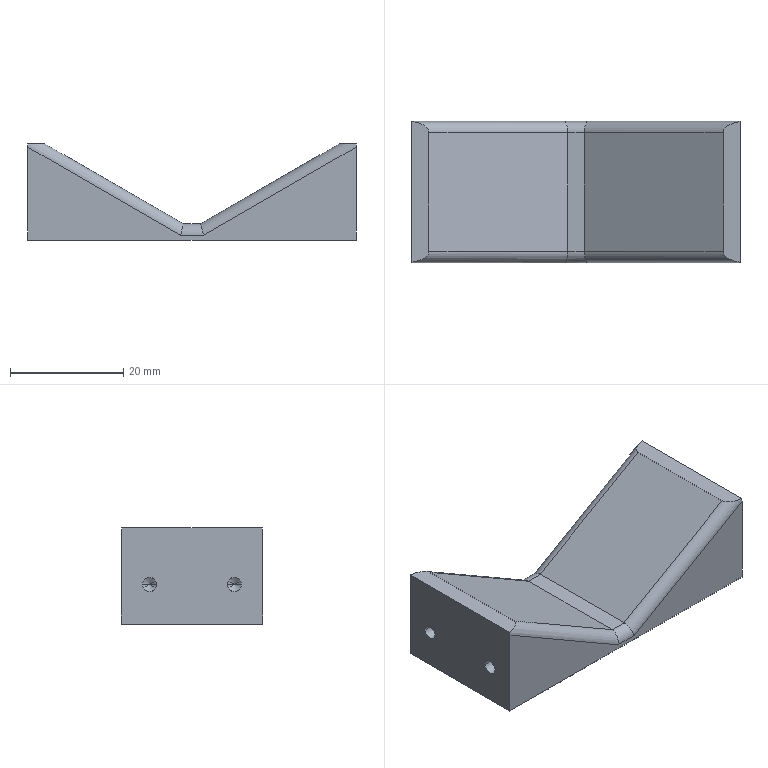CAM job | NX | 3-axis milling | part box 58 x 25 x 17 mm | stock box 64 x 29 x 18 mm
Tools:
number,name,description,diameter,corner_radius,flute_length,length,flutes
1,D63,Milling Tool-5 Parameters,63.0,0.0,50.0,75.0,2
10,D10,Milling Tool-5 Parameters,10.0,0.0,50.0,75.0,2
11,D10JING,Milling Tool-5 Parameters,10.0,0.0,50.0,75.0,2
4,D4,Milling Tool-5 Parameters,4.0,0.0,50.0,75.0,2
5,D3R0.5,Milling Tool-5 Parameters,3.0,0.5,50.0,75.0,2
7,D6A45,Milling Tool-5 Parameters,6.0,0.0,3.0,3.0,2
Operations:
program,operation,operation_type,tool,method,geometry_group,spindle_rpm,surface_speed,feed_per_tooth,feed_cut,feed_plunge,cut_length_mm,path_length_mm,cut_time_min,machine_time_min
1-61-25-20毛胚-虎钳,FLOOR_WALL,VolumeBased25DMillingOperation,D63,METHOD,A,6500.0,1286.0,0.0962,1250.0,100.0,139.0,159.0,0.1112,0.1132
1-61-25-20毛胚-虎钳,ADAPTIVE_MILLING,CavityMilling,D10,METHOD,A,7000.0,219.0,0.2143,3000.0,1000.0,8758.565,14218.255,3.135,3.682
1-61-25-20毛胚-虎钳,ZLEVEL_PROFILE_COPY_COPY_1,ZLevelMilling,D10JING,METHOD,A,7000.0,219.0,0.0714,1000.0,100.0,209.308,265.308,0.2093,0.2149
1-61-25-20毛胚-虎钳,ZLEVEL_PROFILE_COPY_1,ZLevelMilling,D4,METHOD,A,7000.0,87.0,0.1071,1500.0,1000.0,235.517,943.535,0.1605,0.2314
1-61-25-20毛胚-虎钳,ZLEVEL_PROFILE_COPY_1_COPY_1_COPY,ZLevelMilling,D3R0.5,METHOD,A,7000.0,65.0,0.1786,2500.0,1000.0,21474.589,21578.645,8.595,8.605
1-61-25-20毛胚-虎钳,ZLEVEL_PROFILE_COPY_1_COPY_1_COPY_COPY,ZLevelMilling,D3R0.5,METHOD,A,7000.0,65.0,0.1786,2500.0,1000.0,890.953,1021.752,0.3598,0.3729
1-61-25-20毛胚-虎钳,ZLEVEL_PROFILE_COPY_1_COPY_COPY_COPY_COPY_2_COPY,ZLevelMilling,D6A45,METHOD,A,7000.0,131.0,0.0714,1000.0,1000.0,68.807,178.709,0.0688,0.0798